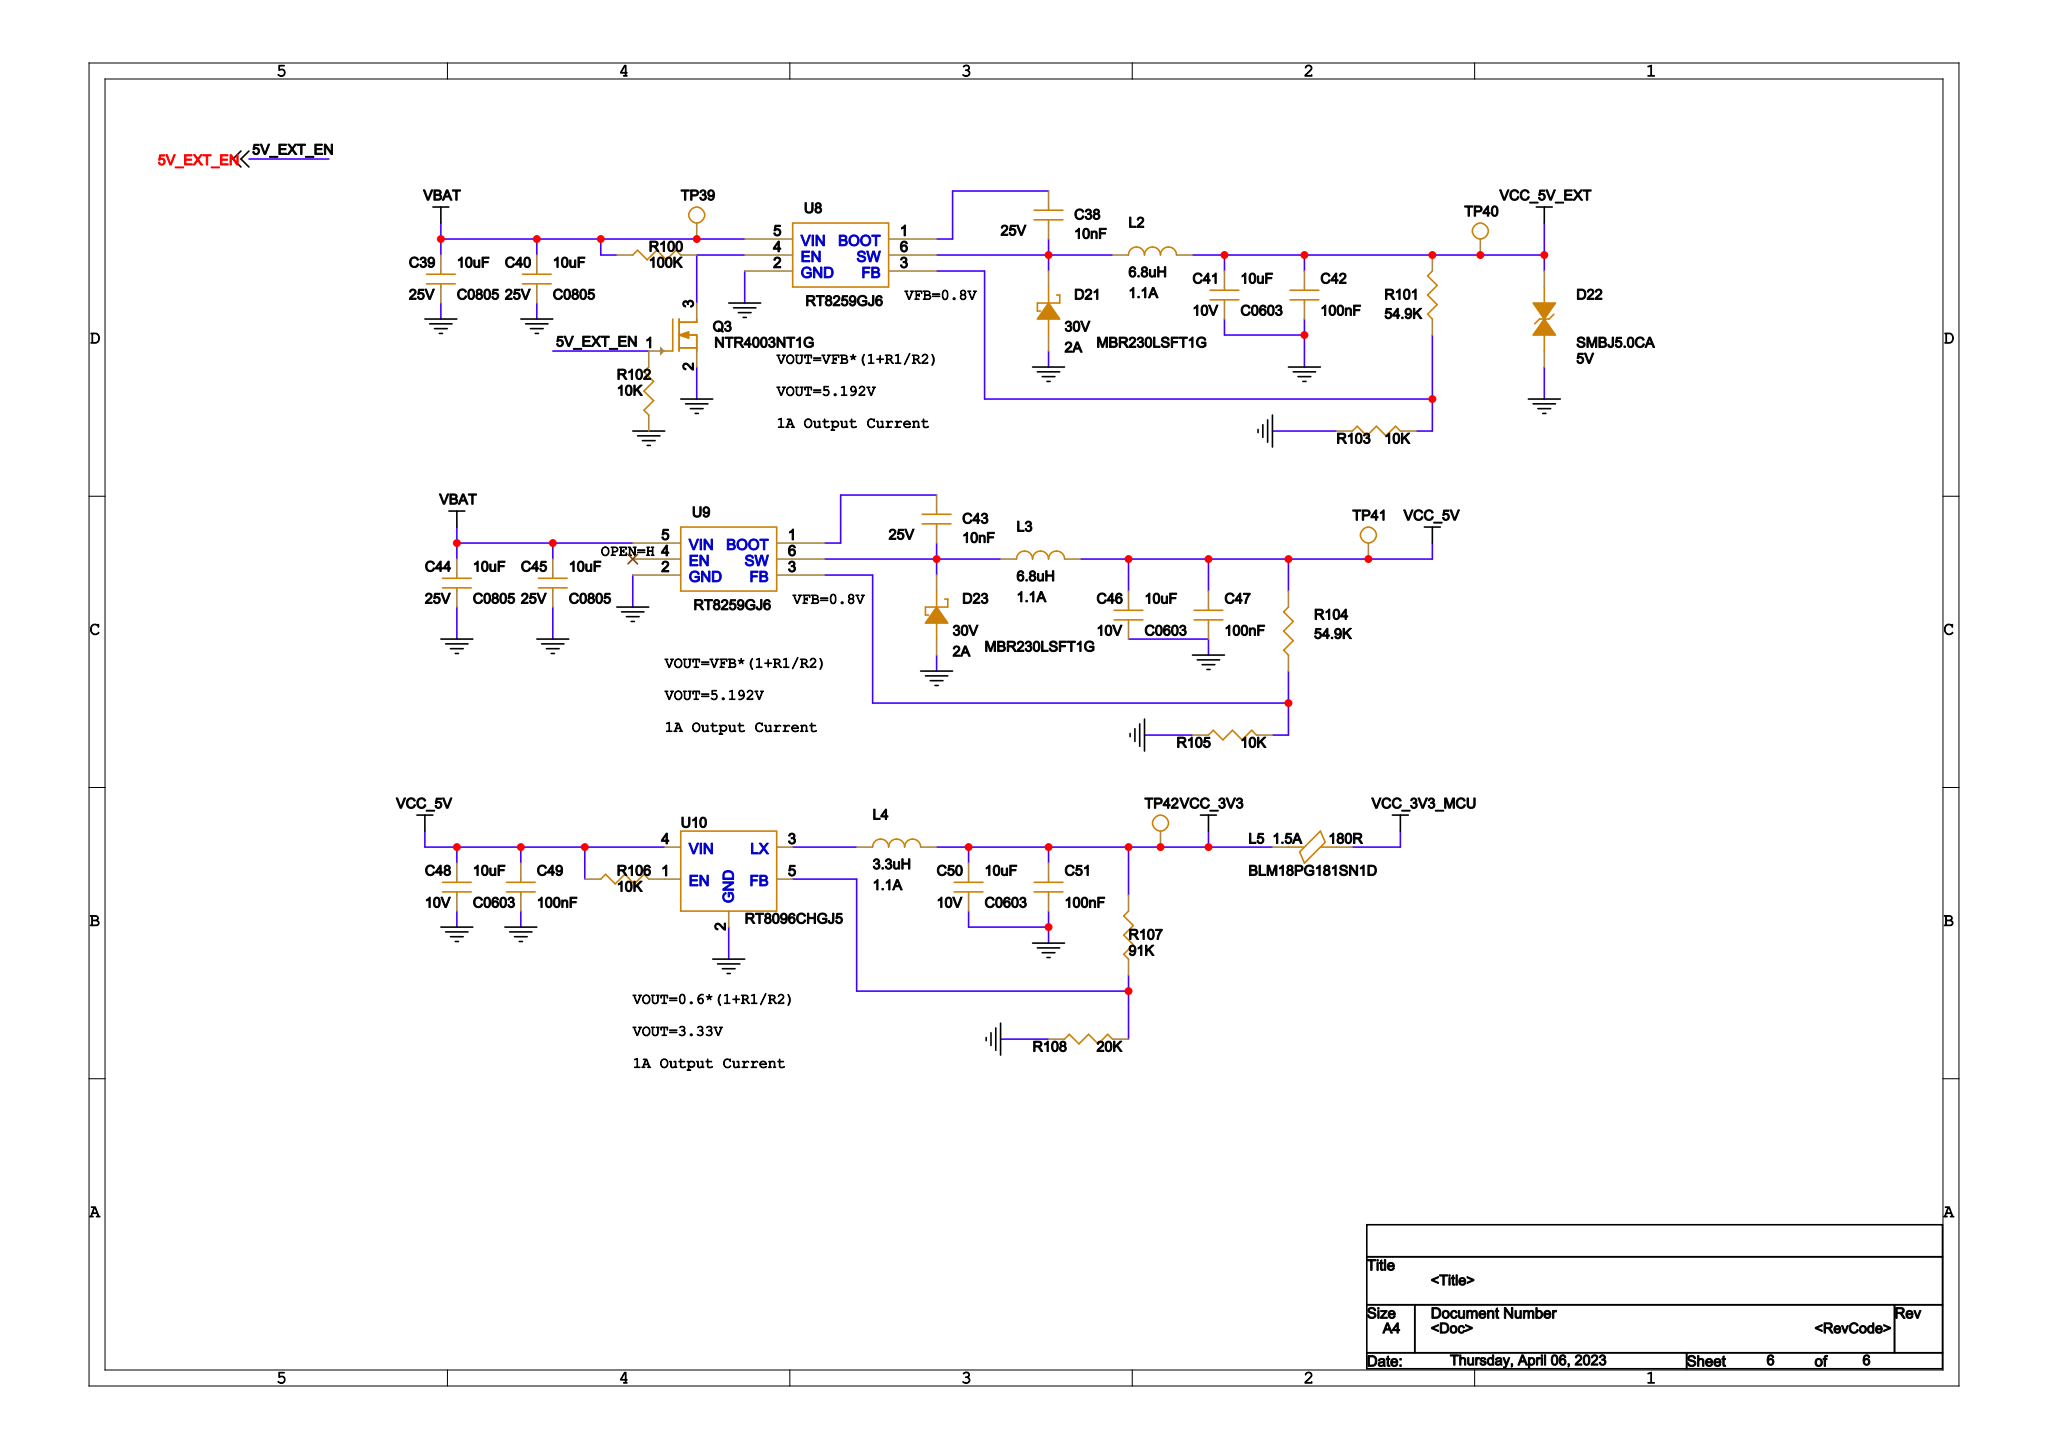Circuit board | Cadence Allegro | 278 parts | 154 nets | one sheet of the schematic
Parts on this sheet (reference | value | footprint):
C38 | 10nF | C0402
C39 | 10uF | C0805
C40 | 10uF | C0805
C41 | 10uF | C0603
C42 | 100nF | C0402
C43 | 10nF | C0402
C44 | 10uF | C0805
C45 | 10uF | C0805
C46 | 10uF | C0603
C47 | 100nF | C0402
C48 | 10uF | C0603
C49 | 100nF | C0402
C50 | 10uF | C0603
C51 | 100nF | C0402
D21 | MBR230LSFT1G | SDO-123F_1
D22 | SMBJ5.0CA | SMBJ18CA
D23 | MBR230LSFT1G | SDO-123F_1
L2 | 6.8uH | LVF303012-6R8M-N
L3 | 6.8uH | LVF303012-6R8M-N
L4 | 3.3uH | LVF303012-3R3M-N
L5 | BLM18PG181SN1D | L0603
Q3 | NTR4003NT1G | SOT-23_0
R100 | 100K | R0402
R101 | 54.9K | R0402
R102 | 10K | R0402
R103 | 10K | R0402
R104 | 54.9K | R0402
R105 | 10K | R0402
R106 | 10K | R0402
R107 | 91K | R0402
R108 | 20K | R0402
TP39 | T POINT R | TP_C1
TP40 | T POINT R | TP_C1
TP41 | T POINT R | TP_C1
TP42 | T POINT R | TP_C1
U8 | RT8259GJ6 | TSOT-23-6
U9 | RT8259GJ6 | TSOT-23-6
U10 | RT8096CHGJ5 | TSOT-23-5
Nets of these parts (net: part-pin ...):
GND: C39-2 C40-2 C41-2 C42-1 C44-2 C45-2 C46-2 C47-1 C48-2 C49-1 C50-2 C51-1 D21-A D22-2 D23-A Q3-2 R102-1 R103-2 R105-2 R108-2 U8-2 U9-2 U10-2
VCC_3V3_MCU: L5-2
VCC_3V3: C50-1 C51-2 L4-2 L5-1 R107-2 TP42-1
VCC_5V_EXT: C41-1 C42-2 D22-1 L2-2 R101-2 TP40-1
VCC_5V: C46-1 C47-2 C48-1 C49-2 L3-2 R104-2 R106-2 TP41-1 U10-4
N16866569: C38-1 U8-1
N16866615: C38-2 D21-K L2-1 U8-6
N16866567: C43-1 U9-1
N16866855: C43-2 D23-K L3-1 U9-6
VBAT: C39-1 C40-1 C44-1 C45-1 R100-1 TP39-1 U8-5 U9-5
N16872080: L4-1 U10-3
N16882854: Q3-3 R100-2 U8-4
5V_EXT_EN: Q3-1 R102-2
N16866711: R101-1 R103-1 U8-3
N16866783: R104-1 R105-1 U9-3
N168715541: R106-1 U10-1
N16873564: R107-1 R108-1 U10-5